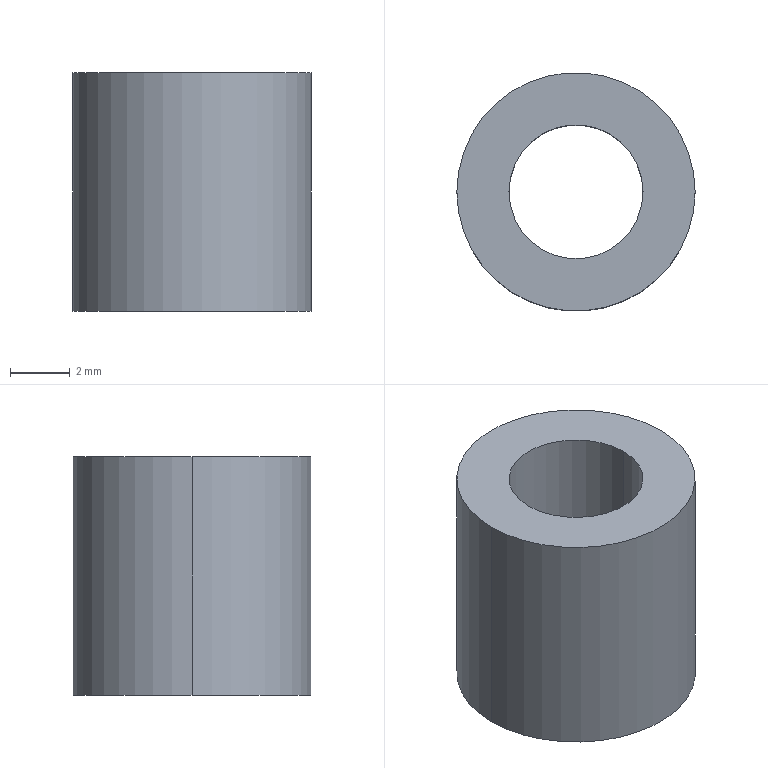Part | STEP file | 02-14 pad block | 1 solid | 6 faces | box 8 x 8 x 8 mm | volume 274.889 mm3 | cylinder 4 | plane 2 | commonest cylinder face diameters 4.5 x2 8 x2
STEP:
#1=CARTESIAN_POINT('',(-2.25,0.,8.));
#2=VERTEX_POINT('',#1);
#3=CARTESIAN_POINT('',(2.25,0.,8.));
#4=VERTEX_POINT('',#3);
#5=CARTESIAN_POINT('',(0.,0.,8.));
#6=DIRECTION('',(0.,0.,1.));
#7=DIRECTION('',(1.,0.,0.));
#8=AXIS2_PLACEMENT_3D('',#5,#6,#7);
#9=CIRCLE('',#8,2.25);
#10=EDGE_CURVE('',#2,#4,#9,.T.);
#11=ORIENTED_EDGE('',*,*,#10,.T.);
#12=CARTESIAN_POINT('',(2.25,0.,0.));
#13=VERTEX_POINT('',#12);
#14=CARTESIAN_POINT('',(2.25,0.,8.));
#15=DIRECTION('',(0.,0.,-1.));
#16=VECTOR('',#15,1000.);
#17=LINE('',#14,#16);
#18=EDGE_CURVE('',#4,#13,#17,.T.);
#19=ORIENTED_EDGE('',*,*,#18,.T.);
#20=CARTESIAN_POINT('',(-2.25,0.,0.));
#21=VERTEX_POINT('',#20);
#22=CARTESIAN_POINT('',(0.,0.,0.));
#23=DIRECTION('',(0.,0.,1.));
#24=DIRECTION('',(1.,0.,0.));
#25=AXIS2_PLACEMENT_3D('',#22,#23,#24);
#26=CIRCLE('',#25,2.25);
#27=EDGE_CURVE('',#21,#13,#26,.T.);
#28=ORIENTED_EDGE('',*,*,#27,.F.);
#29=CARTESIAN_POINT('',(-2.25,0.,8.));
#30=DIRECTION('',(0.,0.,-1.));
#31=VECTOR('',#30,1000.);
#32=LINE('',#29,#31);
#33=EDGE_CURVE('',#2,#21,#32,.T.);
#34=ORIENTED_EDGE('',*,*,#33,.F.);
#35=EDGE_LOOP('',(#11,#19,#28,#34));
#36=FACE_OUTER_BOUND('',#35,.T.);
#37=CARTESIAN_POINT('',(0.,0.,8.));
#38=DIRECTION('',(0.,0.,-1.));
#39=DIRECTION('',(-1.,0.,0.));
#40=AXIS2_PLACEMENT_3D('',#37,#38,#39);
#41=CYLINDRICAL_SURFACE('',#40,2.25);
#42=ADVANCED_FACE('',(#36),#41,.F.);
#43=CARTESIAN_POINT('',(4.,0.,8.));
#44=VERTEX_POINT('',#43);
#45=CARTESIAN_POINT('',(-4.,0.,8.));
#46=VERTEX_POINT('',#45);
#47=CARTESIAN_POINT('',(0.,0.,8.));
#48=DIRECTION('',(0.,0.,1.));
#49=DIRECTION('',(1.,0.,0.));
#50=AXIS2_PLACEMENT_3D('',#47,#48,#49);
#51=CIRCLE('',#50,4.);
#52=EDGE_CURVE('',#44,#46,#51,.T.);
#53=ORIENTED_EDGE('',*,*,#52,.F.);
#54=CARTESIAN_POINT('',(4.,0.,0.));
#55=VERTEX_POINT('',#54);
#56=CARTESIAN_POINT('',(4.,0.,8.));
#57=DIRECTION('',(0.,0.,-1.));
#58=VECTOR('',#57,1000.);
#59=LINE('',#56,#58);
#60=EDGE_CURVE('',#44,#55,#59,.T.);
#61=ORIENTED_EDGE('',*,*,#60,.T.);
#62=CARTESIAN_POINT('',(-4.,0.,0.));
#63=VERTEX_POINT('',#62);
#64=CARTESIAN_POINT('',(0.,0.,0.));
#65=DIRECTION('',(0.,0.,1.));
#66=DIRECTION('',(1.,0.,0.));
#67=AXIS2_PLACEMENT_3D('',#64,#65,#66);
#68=CIRCLE('',#67,4.);
#69=EDGE_CURVE('',#55,#63,#68,.T.);
#70=ORIENTED_EDGE('',*,*,#69,.T.);
#71=CARTESIAN_POINT('',(-4.,0.,8.));
#72=DIRECTION('',(0.,0.,-1.));
#73=VECTOR('',#72,1000.);
#74=LINE('',#71,#73);
#75=EDGE_CURVE('',#46,#63,#74,.T.);
#76=ORIENTED_EDGE('',*,*,#75,.F.);
#77=EDGE_LOOP('',(#53,#61,#70,#76));
#78=FACE_OUTER_BOUND('',#77,.T.);
#79=CARTESIAN_POINT('',(0.,0.,8.));
#80=DIRECTION('',(0.,0.,-1.));
#81=DIRECTION('',(-1.,0.,0.));
#82=AXIS2_PLACEMENT_3D('',#79,#80,#81);
#83=CYLINDRICAL_SURFACE('',#82,4.);
#84=ADVANCED_FACE('',(#78),#83,.T.);
#85=CARTESIAN_POINT('',(0.,0.,8.));
#86=DIRECTION('',(0.,0.,1.));
#87=DIRECTION('',(1.,0.,0.));
#88=AXIS2_PLACEMENT_3D('',#85,#86,#87);
#89=CIRCLE('',#88,4.);
#90=EDGE_CURVE('',#46,#44,#89,.T.);
#91=ORIENTED_EDGE('',*,*,#90,.T.);
#92=ORIENTED_EDGE('',*,*,#52,.T.);
#93=EDGE_LOOP('',(#91,#92));
#94=FACE_OUTER_BOUND('',#93,.T.);
#95=ORIENTED_EDGE('',*,*,#10,.F.);
#96=CARTESIAN_POINT('',(0.,0.,8.));
#97=DIRECTION('',(0.,0.,1.));
#98=DIRECTION('',(1.,0.,0.));
#99=AXIS2_PLACEMENT_3D('',#96,#97,#98);
#100=CIRCLE('',#99,2.25);
#101=EDGE_CURVE('',#4,#2,#100,.T.);
#102=ORIENTED_EDGE('',*,*,#101,.F.);
#103=EDGE_LOOP('',(#95,#102));
#104=FACE_BOUND('',#103,.T.);
#105=CARTESIAN_POINT('',(0.,0.,8.));
#106=DIRECTION('',(0.,0.,1.));
#107=DIRECTION('',(1.,0.,0.));
#108=AXIS2_PLACEMENT_3D('',#105,#106,#107);
#109=PLANE('',#108);
#110=ADVANCED_FACE('',(#94,#104),#109,.T.);
#111=CARTESIAN_POINT('',(0.,0.,0.));
#112=DIRECTION('',(0.,0.,1.));
#113=DIRECTION('',(1.,0.,0.));
#114=AXIS2_PLACEMENT_3D('',#111,#112,#113);
#115=CIRCLE('',#114,4.);
#116=EDGE_CURVE('',#63,#55,#115,.T.);
#117=ORIENTED_EDGE('',*,*,#116,.F.);
#118=ORIENTED_EDGE('',*,*,#69,.F.);
#119=EDGE_LOOP('',(#117,#118));
#120=FACE_OUTER_BOUND('',#119,.T.);
#121=ORIENTED_EDGE('',*,*,#27,.T.);
#122=CARTESIAN_POINT('',(0.,0.,0.));
#123=DIRECTION('',(0.,0.,1.));
#124=DIRECTION('',(1.,0.,0.));
#125=AXIS2_PLACEMENT_3D('',#122,#123,#124);
#126=CIRCLE('',#125,2.25);
#127=EDGE_CURVE('',#13,#21,#126,.T.);
#128=ORIENTED_EDGE('',*,*,#127,.T.);
#129=EDGE_LOOP('',(#121,#128));
#130=FACE_BOUND('',#129,.T.);
#131=CARTESIAN_POINT('',(0.,0.,0.));
#132=DIRECTION('',(0.,0.,1.));
#133=DIRECTION('',(1.,0.,0.));
#134=AXIS2_PLACEMENT_3D('',#131,#132,#133);
#135=PLANE('',#134);
#136=ADVANCED_FACE('',(#120,#130),#135,.F.);
#137=ORIENTED_EDGE('',*,*,#60,.F.);
#138=ORIENTED_EDGE('',*,*,#90,.F.);
#139=ORIENTED_EDGE('',*,*,#75,.T.);
#140=ORIENTED_EDGE('',*,*,#116,.T.);
#141=EDGE_LOOP('',(#137,#138,#139,#140));
#142=FACE_OUTER_BOUND('',#141,.T.);
#143=CARTESIAN_POINT('',(0.,0.,8.));
#144=DIRECTION('',(0.,0.,-1.));
#145=DIRECTION('',(-1.,0.,0.));
#146=AXIS2_PLACEMENT_3D('',#143,#144,#145);
#147=CYLINDRICAL_SURFACE('',#146,4.);
#148=ADVANCED_FACE('',(#142),#147,.T.);
#149=ORIENTED_EDGE('',*,*,#18,.F.);
#150=ORIENTED_EDGE('',*,*,#101,.T.);
#151=ORIENTED_EDGE('',*,*,#33,.T.);
#152=ORIENTED_EDGE('',*,*,#127,.F.);
#153=EDGE_LOOP('',(#149,#150,#151,#152));
#154=FACE_OUTER_BOUND('',#153,.T.);
#155=CARTESIAN_POINT('',(0.,0.,8.));
#156=DIRECTION('',(0.,0.,-1.));
#157=DIRECTION('',(-1.,0.,0.));
#158=AXIS2_PLACEMENT_3D('',#155,#156,#157);
#159=CYLINDRICAL_SURFACE('',#158,2.25);
#160=ADVANCED_FACE('',(#154),#159,.F.);
#161=CLOSED_SHELL('',(#42,#84,#110,#136,#148,#160));
#162=MANIFOLD_SOLID_BREP('',#161);
#163=CARTESIAN_POINT('',(0.,0.,0.));
#164=DIRECTION('',(0.,0.,1.));
#165=DIRECTION('',(1.,0.,0.));
#166=AXIS2_PLACEMENT_3D('',#163,#164,#165);
#167=(LENGTH_UNIT()NAMED_UNIT(*)SI_UNIT(.MILLI.,.METRE.));
#168=UNCERTAINTY_MEASURE_WITH_UNIT(LENGTH_MEASURE(0.00001),#167,'','');
#169=(NAMED_UNIT(*)PLANE_ANGLE_UNIT()SI_UNIT($,.RADIAN.));
#170=(NAMED_UNIT(*)SI_UNIT($,.STERADIAN.)SOLID_ANGLE_UNIT());
#171=(GEOMETRIC_REPRESENTATION_CONTEXT(3)GLOBAL_UNCERTAINTY_ASSIGNED_CONTEXT((#168))GLOBAL_UNIT_ASSIGNED_CONTEXT((#167,#169,#170))REPRESENTATION_CONTEXT('',''));
#172=ADVANCED_BREP_SHAPE_REPRESENTATION('',(#162,#166),#171);